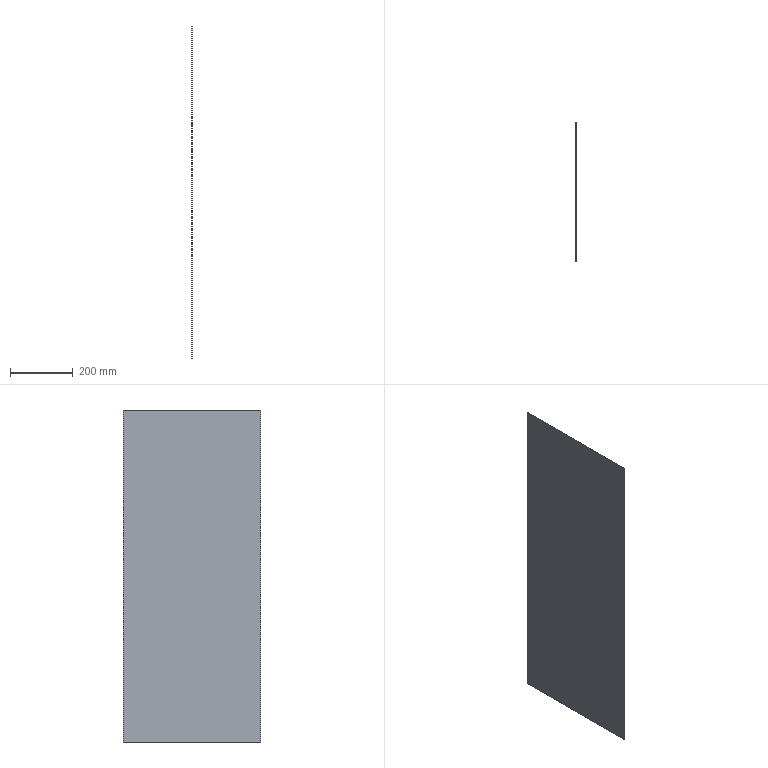Part | SolidWorks | features FlatPattern 1, SMBaseFlange 1, SheetMetal 1 | 1 solid | 6 faces | box 1.2 x 437.6 x 1055 mm | volume 554002 mm3 | plane 6
STEP:
#1=CARTESIAN_POINT('',(153.598,157.841,-527.5));
#2=VERTEX_POINT('',#1);
#3=CARTESIAN_POINT('',(153.598,595.441,-527.5));
#4=VERTEX_POINT('',#3);
#5=CARTESIAN_POINT('',(153.598,157.841,-527.5));
#6=DIRECTION('',(0.,1.,0.));
#7=VECTOR('',#6,1000.);
#8=LINE('',#5,#7);
#9=EDGE_CURVE('',#2,#4,#8,.T.);
#10=ORIENTED_EDGE('',*,*,#9,.T.);
#11=CARTESIAN_POINT('',(153.598,595.441,527.5));
#12=VERTEX_POINT('',#11);
#13=CARTESIAN_POINT('',(153.598,595.441,527.5));
#14=DIRECTION('',(0.,0.,-1.));
#15=VECTOR('',#14,1000.);
#16=LINE('',#13,#15);
#17=EDGE_CURVE('',#12,#4,#16,.T.);
#18=ORIENTED_EDGE('',*,*,#17,.F.);
#19=CARTESIAN_POINT('',(153.598,157.841,527.5));
#20=VERTEX_POINT('',#19);
#21=CARTESIAN_POINT('',(153.598,157.841,527.5));
#22=DIRECTION('',(0.,1.,0.));
#23=VECTOR('',#22,1000.);
#24=LINE('',#21,#23);
#25=EDGE_CURVE('',#20,#12,#24,.T.);
#26=ORIENTED_EDGE('',*,*,#25,.F.);
#27=CARTESIAN_POINT('',(153.598,157.841,527.5));
#28=DIRECTION('',(0.,0.,-1.));
#29=VECTOR('',#28,1000.);
#30=LINE('',#27,#29);
#31=EDGE_CURVE('',#20,#2,#30,.T.);
#32=ORIENTED_EDGE('',*,*,#31,.T.);
#33=EDGE_LOOP('',(#10,#18,#26,#32));
#34=FACE_OUTER_BOUND('',#33,.T.);
#35=CARTESIAN_POINT('',(153.598,157.841,527.5));
#36=DIRECTION('',(-1.,0.,0.));
#37=DIRECTION('',(0.,0.,1.));
#38=AXIS2_PLACEMENT_3D('',#35,#36,#37);
#39=PLANE('',#38);
#40=ADVANCED_FACE('',(#34),#39,.F.);
#41=CARTESIAN_POINT('',(152.398,595.441,-527.5));
#42=VERTEX_POINT('',#41);
#43=CARTESIAN_POINT('',(152.398,595.441,-527.5));
#44=DIRECTION('',(1.,0.,0.));
#45=VECTOR('',#44,1000.);
#46=LINE('',#43,#45);
#47=EDGE_CURVE('',#42,#4,#46,.T.);
#48=ORIENTED_EDGE('',*,*,#47,.F.);
#49=CARTESIAN_POINT('',(152.398,595.441,527.5));
#50=VERTEX_POINT('',#49);
#51=CARTESIAN_POINT('',(152.398,595.441,527.5));
#52=DIRECTION('',(0.,0.,-1.));
#53=VECTOR('',#52,1000.);
#54=LINE('',#51,#53);
#55=EDGE_CURVE('',#50,#42,#54,.T.);
#56=ORIENTED_EDGE('',*,*,#55,.F.);
#57=CARTESIAN_POINT('',(152.398,595.441,527.5));
#58=DIRECTION('',(1.,0.,0.));
#59=VECTOR('',#58,1000.);
#60=LINE('',#57,#59);
#61=EDGE_CURVE('',#50,#12,#60,.T.);
#62=ORIENTED_EDGE('',*,*,#61,.T.);
#63=ORIENTED_EDGE('',*,*,#17,.T.);
#64=EDGE_LOOP('',(#48,#56,#62,#63));
#65=FACE_OUTER_BOUND('',#64,.T.);
#66=CARTESIAN_POINT('',(152.398,595.441,527.5));
#67=DIRECTION('',(0.,1.,0.));
#68=DIRECTION('',(0.,0.,1.));
#69=AXIS2_PLACEMENT_3D('',#66,#67,#68);
#70=PLANE('',#69);
#71=ADVANCED_FACE('',(#65),#70,.T.);
#72=CARTESIAN_POINT('',(152.398,157.841,-527.5));
#73=VERTEX_POINT('',#72);
#74=CARTESIAN_POINT('',(152.398,157.841,-527.5));
#75=DIRECTION('',(0.,1.,0.));
#76=VECTOR('',#75,1000.);
#77=LINE('',#74,#76);
#78=EDGE_CURVE('',#73,#42,#77,.T.);
#79=ORIENTED_EDGE('',*,*,#78,.F.);
#80=CARTESIAN_POINT('',(152.398,157.841,527.5));
#81=VERTEX_POINT('',#80);
#82=CARTESIAN_POINT('',(152.398,157.841,527.5));
#83=DIRECTION('',(0.,0.,-1.));
#84=VECTOR('',#83,1000.);
#85=LINE('',#82,#84);
#86=EDGE_CURVE('',#81,#73,#85,.T.);
#87=ORIENTED_EDGE('',*,*,#86,.F.);
#88=CARTESIAN_POINT('',(152.398,157.841,527.5));
#89=DIRECTION('',(0.,1.,0.));
#90=VECTOR('',#89,1000.);
#91=LINE('',#88,#90);
#92=EDGE_CURVE('',#81,#50,#91,.T.);
#93=ORIENTED_EDGE('',*,*,#92,.T.);
#94=ORIENTED_EDGE('',*,*,#55,.T.);
#95=EDGE_LOOP('',(#79,#87,#93,#94));
#96=FACE_OUTER_BOUND('',#95,.T.);
#97=CARTESIAN_POINT('',(152.398,157.841,527.5));
#98=DIRECTION('',(-1.,0.,0.));
#99=DIRECTION('',(0.,0.,1.));
#100=AXIS2_PLACEMENT_3D('',#97,#98,#99);
#101=PLANE('',#100);
#102=ADVANCED_FACE('',(#96),#101,.T.);
#103=CARTESIAN_POINT('',(153.598,157.841,-527.5));
#104=DIRECTION('',(-1.,0.,0.));
#105=VECTOR('',#104,1000.);
#106=LINE('',#103,#105);
#107=EDGE_CURVE('',#2,#73,#106,.T.);
#108=ORIENTED_EDGE('',*,*,#107,.F.);
#109=ORIENTED_EDGE('',*,*,#31,.F.);
#110=CARTESIAN_POINT('',(153.598,157.841,527.5));
#111=DIRECTION('',(-1.,0.,0.));
#112=VECTOR('',#111,1000.);
#113=LINE('',#110,#112);
#114=EDGE_CURVE('',#20,#81,#113,.T.);
#115=ORIENTED_EDGE('',*,*,#114,.T.);
#116=ORIENTED_EDGE('',*,*,#86,.T.);
#117=EDGE_LOOP('',(#108,#109,#115,#116));
#118=FACE_OUTER_BOUND('',#117,.T.);
#119=CARTESIAN_POINT('',(153.598,157.841,527.5));
#120=DIRECTION('',(0.,-1.,0.));
#121=DIRECTION('',(0.,0.,-1.));
#122=AXIS2_PLACEMENT_3D('',#119,#120,#121);
#123=PLANE('',#122);
#124=ADVANCED_FACE('',(#118),#123,.T.);
#125=ORIENTED_EDGE('',*,*,#25,.T.);
#126=ORIENTED_EDGE('',*,*,#61,.F.);
#127=ORIENTED_EDGE('',*,*,#92,.F.);
#128=ORIENTED_EDGE('',*,*,#114,.F.);
#129=EDGE_LOOP('',(#125,#126,#127,#128));
#130=FACE_OUTER_BOUND('',#129,.T.);
#131=CARTESIAN_POINT('',(0.,0.,527.5));
#132=DIRECTION('',(0.,0.,-1.));
#133=DIRECTION('',(-1.,0.,0.));
#134=AXIS2_PLACEMENT_3D('',#131,#132,#133);
#135=PLANE('',#134);
#136=ADVANCED_FACE('',(#130),#135,.F.);
#137=ORIENTED_EDGE('',*,*,#9,.F.);
#138=ORIENTED_EDGE('',*,*,#107,.T.);
#139=ORIENTED_EDGE('',*,*,#78,.T.);
#140=ORIENTED_EDGE('',*,*,#47,.T.);
#141=EDGE_LOOP('',(#137,#138,#139,#140));
#142=FACE_OUTER_BOUND('',#141,.T.);
#143=CARTESIAN_POINT('',(0.,0.,-527.5));
#144=DIRECTION('',(0.,0.,-1.));
#145=DIRECTION('',(-1.,0.,0.));
#146=AXIS2_PLACEMENT_3D('',#143,#144,#145);
#147=PLANE('',#146);
#148=ADVANCED_FACE('',(#142),#147,.T.);
#149=CLOSED_SHELL('',(#40,#71,#102,#124,#136,#148));
#150=MANIFOLD_SOLID_BREP('',#149);
#151=CARTESIAN_POINT('',(0.,0.,0.));
#152=DIRECTION('',(0.,0.,1.));
#153=DIRECTION('',(1.,0.,0.));
#154=AXIS2_PLACEMENT_3D('',#151,#152,#153);
#155=(LENGTH_UNIT()NAMED_UNIT(*)SI_UNIT(.MILLI.,.METRE.));
#156=UNCERTAINTY_MEASURE_WITH_UNIT(LENGTH_MEASURE(0.00001),#155,'','');
#157=(NAMED_UNIT(*)PLANE_ANGLE_UNIT()SI_UNIT($,.RADIAN.));
#158=(NAMED_UNIT(*)SI_UNIT($,.STERADIAN.)SOLID_ANGLE_UNIT());
#159=(GEOMETRIC_REPRESENTATION_CONTEXT(3)GLOBAL_UNCERTAINTY_ASSIGNED_CONTEXT((#156))GLOBAL_UNIT_ASSIGNED_CONTEXT((#155,#157,#158))REPRESENTATION_CONTEXT('',''));
#160=ADVANCED_BREP_SHAPE_REPRESENTATION('',(#150,#154),#159);